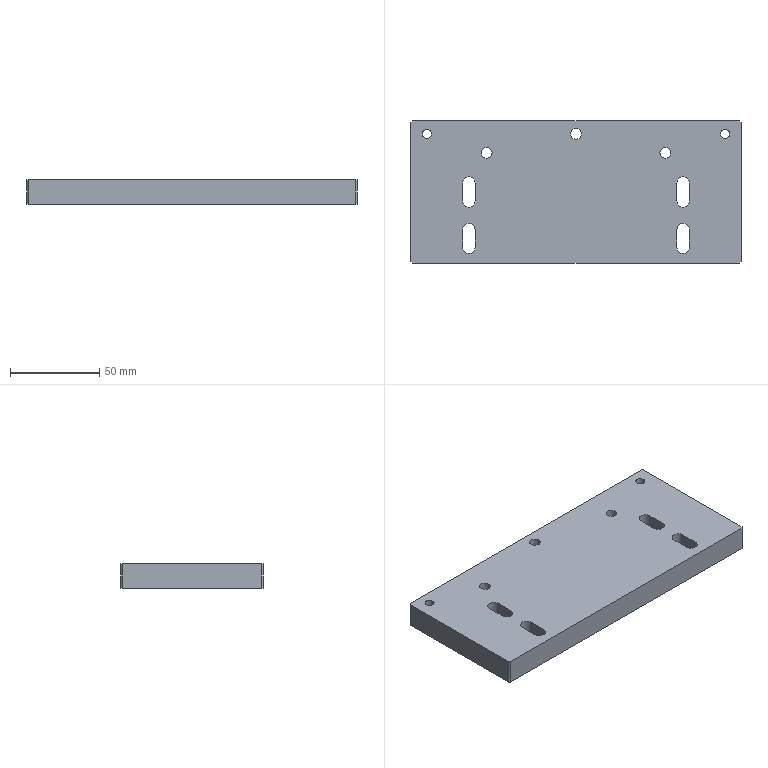Part | NX | 1 solid | 31 faces | box 185 x 80 x 14 mm | volume 199360 mm3 | plane 18 | cylinder 13 | commonest cylinder face diameters 7 x8 6 x3 5 x2
STEP:
#1=CARTESIAN_POINT('',(-91.5,40.,7.));
#2=VERTEX_POINT('',#1);
#3=CARTESIAN_POINT('',(-92.5,39.,7.));
#4=VERTEX_POINT('',#3);
#5=CARTESIAN_POINT('',(-65.75,65.75,7.));
#6=DIRECTION('',(-0.7071,-0.7071,0.));
#7=VECTOR('',#6,1000.);
#8=LINE('',#5,#7);
#9=EDGE_CURVE('',#2,#4,#8,.T.);
#10=ORIENTED_EDGE('',*,*,#9,.F.);
#11=CARTESIAN_POINT('',(-91.5,40.,-7.));
#12=VERTEX_POINT('',#11);
#13=CARTESIAN_POINT('',(-91.5,40.,7.));
#14=DIRECTION('',(0.,0.,1.));
#15=VECTOR('',#14,1000.);
#16=LINE('',#13,#15);
#17=EDGE_CURVE('',#12,#2,#16,.T.);
#18=ORIENTED_EDGE('',*,*,#17,.F.);
#19=CARTESIAN_POINT('',(-92.5,39.,-7.));
#20=VERTEX_POINT('',#19);
#21=CARTESIAN_POINT('',(-92.5,39.,-7.));
#22=DIRECTION('',(0.7071,0.7071,0.));
#23=VECTOR('',#22,1000.);
#24=LINE('',#21,#23);
#25=EDGE_CURVE('',#20,#12,#24,.T.);
#26=ORIENTED_EDGE('',*,*,#25,.F.);
#27=CARTESIAN_POINT('',(-92.5,39.,7.));
#28=DIRECTION('',(0.,0.,-1.));
#29=VECTOR('',#28,1000.);
#30=LINE('',#27,#29);
#31=EDGE_CURVE('',#4,#20,#30,.T.);
#32=ORIENTED_EDGE('',*,*,#31,.F.);
#33=EDGE_LOOP('',(#10,#18,#26,#32));
#34=FACE_BOUND('',#33,.T.);
#35=CARTESIAN_POINT('',(-92.5,39.,7.));
#36=DIRECTION('',(0.7071,-0.7071,0.));
#37=DIRECTION('',(0.,0.,-1.));
#38=AXIS2_PLACEMENT_3D('',#35,#36,#37);
#39=PLANE('',#38);
#40=ADVANCED_FACE('',(#34),#39,.F.);
#41=CARTESIAN_POINT('',(-92.5,-39.,7.));
#42=VERTEX_POINT('',#41);
#43=CARTESIAN_POINT('',(-91.5,-40.,7.));
#44=VERTEX_POINT('',#43);
#45=CARTESIAN_POINT('',(-65.75,-65.75,7.));
#46=DIRECTION('',(0.7071,-0.7071,0.));
#47=VECTOR('',#46,1000.);
#48=LINE('',#45,#47);
#49=EDGE_CURVE('',#42,#44,#48,.T.);
#50=ORIENTED_EDGE('',*,*,#49,.F.);
#51=CARTESIAN_POINT('',(-92.5,-39.,-7.));
#52=VERTEX_POINT('',#51);
#53=CARTESIAN_POINT('',(-92.5,-39.,7.));
#54=DIRECTION('',(0.,0.,1.));
#55=VECTOR('',#54,1000.);
#56=LINE('',#53,#55);
#57=EDGE_CURVE('',#52,#42,#56,.T.);
#58=ORIENTED_EDGE('',*,*,#57,.F.);
#59=CARTESIAN_POINT('',(-91.5,-40.,-7.));
#60=VERTEX_POINT('',#59);
#61=CARTESIAN_POINT('',(-91.5,-40.,-7.));
#62=DIRECTION('',(-0.7071,0.7071,0.));
#63=VECTOR('',#62,1000.);
#64=LINE('',#61,#63);
#65=EDGE_CURVE('',#60,#52,#64,.T.);
#66=ORIENTED_EDGE('',*,*,#65,.F.);
#67=CARTESIAN_POINT('',(-91.5,-40.,7.));
#68=DIRECTION('',(0.,0.,-1.));
#69=VECTOR('',#68,1000.);
#70=LINE('',#67,#69);
#71=EDGE_CURVE('',#44,#60,#70,.T.);
#72=ORIENTED_EDGE('',*,*,#71,.F.);
#73=EDGE_LOOP('',(#50,#58,#66,#72));
#74=FACE_BOUND('',#73,.T.);
#75=CARTESIAN_POINT('',(-91.5,-40.,7.));
#76=DIRECTION('',(0.7071,0.7071,0.));
#77=DIRECTION('',(0.,0.,-1.));
#78=AXIS2_PLACEMENT_3D('',#75,#76,#77);
#79=PLANE('',#78);
#80=ADVANCED_FACE('',(#74),#79,.F.);
#81=CARTESIAN_POINT('',(91.5,-40.,7.));
#82=VERTEX_POINT('',#81);
#83=CARTESIAN_POINT('',(92.5,-39.,7.));
#84=VERTEX_POINT('',#83);
#85=CARTESIAN_POINT('',(65.75,-65.75,7.));
#86=DIRECTION('',(0.7071,0.7071,0.));
#87=VECTOR('',#86,1000.);
#88=LINE('',#85,#87);
#89=EDGE_CURVE('',#82,#84,#88,.T.);
#90=ORIENTED_EDGE('',*,*,#89,.F.);
#91=CARTESIAN_POINT('',(91.5,-40.,-7.));
#92=VERTEX_POINT('',#91);
#93=CARTESIAN_POINT('',(91.5,-40.,7.));
#94=DIRECTION('',(0.,0.,1.));
#95=VECTOR('',#94,1000.);
#96=LINE('',#93,#95);
#97=EDGE_CURVE('',#92,#82,#96,.T.);
#98=ORIENTED_EDGE('',*,*,#97,.F.);
#99=CARTESIAN_POINT('',(92.5,-39.,-7.));
#100=VERTEX_POINT('',#99);
#101=CARTESIAN_POINT('',(92.5,-39.,-7.));
#102=DIRECTION('',(-0.7071,-0.7071,0.));
#103=VECTOR('',#102,1000.);
#104=LINE('',#101,#103);
#105=EDGE_CURVE('',#100,#92,#104,.T.);
#106=ORIENTED_EDGE('',*,*,#105,.F.);
#107=CARTESIAN_POINT('',(92.5,-39.,7.));
#108=DIRECTION('',(0.,0.,-1.));
#109=VECTOR('',#108,1000.);
#110=LINE('',#107,#109);
#111=EDGE_CURVE('',#84,#100,#110,.T.);
#112=ORIENTED_EDGE('',*,*,#111,.F.);
#113=EDGE_LOOP('',(#90,#98,#106,#112));
#114=FACE_BOUND('',#113,.T.);
#115=CARTESIAN_POINT('',(92.5,-39.,7.));
#116=DIRECTION('',(-0.7071,0.7071,0.));
#117=DIRECTION('',(0.,0.,-1.));
#118=AXIS2_PLACEMENT_3D('',#115,#116,#117);
#119=PLANE('',#118);
#120=ADVANCED_FACE('',(#114),#119,.F.);
#121=CARTESIAN_POINT('',(92.5,39.,7.));
#122=VERTEX_POINT('',#121);
#123=CARTESIAN_POINT('',(91.5,40.,7.));
#124=VERTEX_POINT('',#123);
#125=CARTESIAN_POINT('',(65.75,65.75,7.));
#126=DIRECTION('',(-0.7071,0.7071,0.));
#127=VECTOR('',#126,1000.);
#128=LINE('',#125,#127);
#129=EDGE_CURVE('',#122,#124,#128,.T.);
#130=ORIENTED_EDGE('',*,*,#129,.F.);
#131=CARTESIAN_POINT('',(92.5,39.,-7.));
#132=VERTEX_POINT('',#131);
#133=CARTESIAN_POINT('',(92.5,39.,7.));
#134=DIRECTION('',(0.,0.,1.));
#135=VECTOR('',#134,1000.);
#136=LINE('',#133,#135);
#137=EDGE_CURVE('',#132,#122,#136,.T.);
#138=ORIENTED_EDGE('',*,*,#137,.F.);
#139=CARTESIAN_POINT('',(91.5,40.,-7.));
#140=VERTEX_POINT('',#139);
#141=CARTESIAN_POINT('',(91.5,40.,-7.));
#142=DIRECTION('',(0.7071,-0.7071,0.));
#143=VECTOR('',#142,1000.);
#144=LINE('',#141,#143);
#145=EDGE_CURVE('',#140,#132,#144,.T.);
#146=ORIENTED_EDGE('',*,*,#145,.F.);
#147=CARTESIAN_POINT('',(91.5,40.,7.));
#148=DIRECTION('',(0.,0.,-1.));
#149=VECTOR('',#148,1000.);
#150=LINE('',#147,#149);
#151=EDGE_CURVE('',#124,#140,#150,.T.);
#152=ORIENTED_EDGE('',*,*,#151,.F.);
#153=EDGE_LOOP('',(#130,#138,#146,#152));
#154=FACE_BOUND('',#153,.T.);
#155=CARTESIAN_POINT('',(91.5,40.,7.));
#156=DIRECTION('',(-0.7071,-0.7071,0.));
#157=DIRECTION('',(0.,0.,-1.));
#158=AXIS2_PLACEMENT_3D('',#155,#156,#157);
#159=PLANE('',#158);
#160=ADVANCED_FACE('',(#154),#159,.F.);
#161=CARTESIAN_POINT('',(-56.5,-21.,7.));
#162=VERTEX_POINT('',#161);
#163=CARTESIAN_POINT('',(-56.5,-21.,-7.));
#164=VERTEX_POINT('',#163);
#165=CARTESIAN_POINT('',(-56.5,-21.,7.));
#166=DIRECTION('',(0.,0.,-1.));
#167=VECTOR('',#166,1000.);
#168=LINE('',#165,#167);
#169=EDGE_CURVE('',#162,#164,#168,.T.);
#170=ORIENTED_EDGE('',*,*,#169,.T.);
#171=CARTESIAN_POINT('',(-56.5,-31.,-7.));
#172=VERTEX_POINT('',#171);
#173=CARTESIAN_POINT('',(-56.5,0.,-7.));
#174=DIRECTION('',(0.,1.,0.));
#175=VECTOR('',#174,1000.);
#176=LINE('',#173,#175);
#177=EDGE_CURVE('',#172,#164,#176,.T.);
#178=ORIENTED_EDGE('',*,*,#177,.F.);
#179=CARTESIAN_POINT('',(-56.5,-31.,7.));
#180=VERTEX_POINT('',#179);
#181=CARTESIAN_POINT('',(-56.5,-31.,7.));
#182=DIRECTION('',(0.,0.,-1.));
#183=VECTOR('',#182,1000.);
#184=LINE('',#181,#183);
#185=EDGE_CURVE('',#180,#172,#184,.T.);
#186=ORIENTED_EDGE('',*,*,#185,.F.);
#187=CARTESIAN_POINT('',(-56.5,-5.,7.));
#188=DIRECTION('',(0.,1.,0.));
#189=VECTOR('',#188,1000.);
#190=LINE('',#187,#189);
#191=EDGE_CURVE('',#180,#162,#190,.T.);
#192=ORIENTED_EDGE('',*,*,#191,.T.);
#193=EDGE_LOOP('',(#170,#178,#186,#192));
#194=FACE_BOUND('',#193,.T.);
#195=CARTESIAN_POINT('',(-56.5,-5.,-7.));
#196=DIRECTION('',(1.,0.,0.));
#197=DIRECTION('',(0.,0.,-1.));
#198=AXIS2_PLACEMENT_3D('',#195,#196,#197);
#199=PLANE('',#198);
#200=ADVANCED_FACE('',(#194),#199,.F.);
#201=CARTESIAN_POINT('',(-63.5,-21.,-7.));
#202=VERTEX_POINT('',#201);
#203=CARTESIAN_POINT('',(-63.5,-21.,7.));
#204=VERTEX_POINT('',#203);
#205=CARTESIAN_POINT('',(-63.5,-21.,7.));
#206=DIRECTION('',(0.,0.,1.));
#207=VECTOR('',#206,1000.);
#208=LINE('',#205,#207);
#209=EDGE_CURVE('',#202,#204,#208,.T.);
#210=ORIENTED_EDGE('',*,*,#209,.T.);
#211=CARTESIAN_POINT('',(-63.5,-31.,7.));
#212=VERTEX_POINT('',#211);
#213=CARTESIAN_POINT('',(-63.5,0.,7.));
#214=DIRECTION('',(0.,1.,0.));
#215=VECTOR('',#214,1000.);
#216=LINE('',#213,#215);
#217=EDGE_CURVE('',#212,#204,#216,.T.);
#218=ORIENTED_EDGE('',*,*,#217,.F.);
#219=CARTESIAN_POINT('',(-63.5,-31.,-7.));
#220=VERTEX_POINT('',#219);
#221=CARTESIAN_POINT('',(-63.5,-31.,7.));
#222=DIRECTION('',(0.,0.,-1.));
#223=VECTOR('',#222,1000.);
#224=LINE('',#221,#223);
#225=EDGE_CURVE('',#212,#220,#224,.T.);
#226=ORIENTED_EDGE('',*,*,#225,.T.);
#227=CARTESIAN_POINT('',(-63.5,-5.,-7.));
#228=DIRECTION('',(0.,1.,0.));
#229=VECTOR('',#228,1000.);
#230=LINE('',#227,#229);
#231=EDGE_CURVE('',#220,#202,#230,.T.);
#232=ORIENTED_EDGE('',*,*,#231,.T.);
#233=EDGE_LOOP('',(#210,#218,#226,#232));
#234=FACE_BOUND('',#233,.T.);
#235=CARTESIAN_POINT('',(-63.5,-5.,7.));
#236=DIRECTION('',(-1.,0.,0.));
#237=DIRECTION('',(0.,0.,1.));
#238=AXIS2_PLACEMENT_3D('',#235,#236,#237);
#239=PLANE('',#238);
#240=ADVANCED_FACE('',(#234),#239,.F.);
#241=CARTESIAN_POINT('',(-60.,-31.,7.));
#242=DIRECTION('',(0.,0.,1.));
#243=DIRECTION('',(1.,0.,0.));
#244=AXIS2_PLACEMENT_3D('',#241,#242,#243);
#245=CIRCLE('',#244,3.5);
#246=EDGE_CURVE('',#212,#180,#245,.T.);
#247=ORIENTED_EDGE('',*,*,#246,.T.);
#248=ORIENTED_EDGE('',*,*,#185,.T.);
#249=CARTESIAN_POINT('',(-60.,-31.,-7.));
#250=DIRECTION('',(0.,0.,1.));
#251=DIRECTION('',(1.,0.,0.));
#252=AXIS2_PLACEMENT_3D('',#249,#250,#251);
#253=CIRCLE('',#252,3.5);
#254=EDGE_CURVE('',#220,#172,#253,.T.);
#255=ORIENTED_EDGE('',*,*,#254,.F.);
#256=ORIENTED_EDGE('',*,*,#225,.F.);
#257=EDGE_LOOP('',(#247,#248,#255,#256));
#258=FACE_BOUND('',#257,.T.);
#259=CARTESIAN_POINT('',(-60.,-31.,7.));
#260=DIRECTION('',(0.,0.,1.));
#261=DIRECTION('',(1.,0.,0.));
#262=AXIS2_PLACEMENT_3D('',#259,#260,#261);
#263=CYLINDRICAL_SURFACE('',#262,3.5);
#264=ADVANCED_FACE('',(#258),#263,.F.);
#265=CARTESIAN_POINT('',(-60.,-21.,-7.));
#266=DIRECTION('',(0.,0.,1.));
#267=DIRECTION('',(1.,0.,0.));
#268=AXIS2_PLACEMENT_3D('',#265,#266,#267);
#269=CIRCLE('',#268,3.5);
#270=EDGE_CURVE('',#164,#202,#269,.T.);
#271=ORIENTED_EDGE('',*,*,#270,.F.);
#272=ORIENTED_EDGE('',*,*,#169,.F.);
#273=CARTESIAN_POINT('',(-60.,-21.,7.));
#274=DIRECTION('',(0.,0.,1.));
#275=DIRECTION('',(1.,0.,0.));
#276=AXIS2_PLACEMENT_3D('',#273,#274,#275);
#277=CIRCLE('',#276,3.5);
#278=EDGE_CURVE('',#162,#204,#277,.T.);
#279=ORIENTED_EDGE('',*,*,#278,.T.);
#280=ORIENTED_EDGE('',*,*,#209,.F.);
#281=EDGE_LOOP('',(#271,#272,#279,#280));
#282=FACE_BOUND('',#281,.T.);
#283=CARTESIAN_POINT('',(-60.,-21.,7.));
#284=DIRECTION('',(0.,0.,1.));
#285=DIRECTION('',(1.,0.,0.));
#286=AXIS2_PLACEMENT_3D('',#283,#284,#285);
#287=CYLINDRICAL_SURFACE('',#286,3.5);
#288=ADVANCED_FACE('',(#282),#287,.F.);
#289=CARTESIAN_POINT('',(-56.5,5.,7.));
#290=VERTEX_POINT('',#289);
#291=CARTESIAN_POINT('',(-56.5,5.,-7.));
#292=VERTEX_POINT('',#291);
#293=CARTESIAN_POINT('',(-56.5,5.,-7.));
#294=DIRECTION('',(0.,0.,-1.));
#295=VECTOR('',#294,1000.);
#296=LINE('',#293,#295);
#297=EDGE_CURVE('',#290,#292,#296,.T.);
#298=ORIENTED_EDGE('',*,*,#297,.T.);
#299=CARTESIAN_POINT('',(-56.5,-5.,-7.));
#300=VERTEX_POINT('',#299);
#301=CARTESIAN_POINT('',(-56.5,-5.,-7.));
#302=DIRECTION('',(0.,1.,0.));
#303=VECTOR('',#302,1000.);
#304=LINE('',#301,#303);
#305=EDGE_CURVE('',#300,#292,#304,.T.);
#306=ORIENTED_EDGE('',*,*,#305,.F.);
#307=CARTESIAN_POINT('',(-56.5,-5.,7.));
#308=VERTEX_POINT('',#307);
#309=CARTESIAN_POINT('',(-56.5,-5.,-7.));
#310=DIRECTION('',(0.,0.,-1.));
#311=VECTOR('',#310,1000.);
#312=LINE('',#309,#311);
#313=EDGE_CURVE('',#308,#300,#312,.T.);
#314=ORIENTED_EDGE('',*,*,#313,.F.);
#315=CARTESIAN_POINT('',(-56.5,-5.,7.));
#316=DIRECTION('',(0.,1.,0.));
#317=VECTOR('',#316,1000.);
#318=LINE('',#315,#317);
#319=EDGE_CURVE('',#308,#290,#318,.T.);
#320=ORIENTED_EDGE('',*,*,#319,.T.);
#321=EDGE_LOOP('',(#298,#306,#314,#320));
#322=FACE_BOUND('',#321,.T.);
#323=CARTESIAN_POINT('',(-56.5,-5.,-7.));
#324=DIRECTION('',(1.,0.,0.));
#325=DIRECTION('',(0.,0.,-1.));
#326=AXIS2_PLACEMENT_3D('',#323,#324,#325);
#327=PLANE('',#326);
#328=ADVANCED_FACE('',(#322),#327,.F.);
#329=CARTESIAN_POINT('',(-63.5,5.,-7.));
#330=VERTEX_POINT('',#329);
#331=CARTESIAN_POINT('',(-63.5,5.,7.));
#332=VERTEX_POINT('',#331);
#333=CARTESIAN_POINT('',(-63.5,5.,7.));
#334=DIRECTION('',(0.,0.,1.));
#335=VECTOR('',#334,1000.);
#336=LINE('',#333,#335);
#337=EDGE_CURVE('',#330,#332,#336,.T.);
#338=ORIENTED_EDGE('',*,*,#337,.T.);
#339=CARTESIAN_POINT('',(-63.5,-5.,7.));
#340=VERTEX_POINT('',#339);
#341=CARTESIAN_POINT('',(-63.5,-5.,7.));
#342=DIRECTION('',(0.,1.,0.));
#343=VECTOR('',#342,1000.);
#344=LINE('',#341,#343);
#345=EDGE_CURVE('',#340,#332,#344,.T.);
#346=ORIENTED_EDGE('',*,*,#345,.F.);
#347=CARTESIAN_POINT('',(-63.5,-5.,-7.));
#348=VERTEX_POINT('',#347);
#349=CARTESIAN_POINT('',(-63.5,-5.,7.));
#350=DIRECTION('',(0.,0.,-1.));
#351=VECTOR('',#350,1000.);
#352=LINE('',#349,#351);
#353=EDGE_CURVE('',#340,#348,#352,.T.);
#354=ORIENTED_EDGE('',*,*,#353,.T.);
#355=CARTESIAN_POINT('',(-63.5,-5.,-7.));
#356=DIRECTION('',(0.,1.,0.));
#357=VECTOR('',#356,1000.);
#358=LINE('',#355,#357);
#359=EDGE_CURVE('',#348,#330,#358,.T.);
#360=ORIENTED_EDGE('',*,*,#359,.T.);
#361=EDGE_LOOP('',(#338,#346,#354,#360));
#362=FACE_BOUND('',#361,.T.);
#363=CARTESIAN_POINT('',(-63.5,-5.,7.));
#364=DIRECTION('',(-1.,0.,0.));
#365=DIRECTION('',(0.,0.,1.));
#366=AXIS2_PLACEMENT_3D('',#363,#364,#365);
#367=PLANE('',#366);
#368=ADVANCED_FACE('',(#362),#367,.F.);
#369=CARTESIAN_POINT('',(-60.,-5.,7.));
#370=DIRECTION('',(0.,0.,1.));
#371=DIRECTION('',(1.,0.,0.));
#372=AXIS2_PLACEMENT_3D('',#369,#370,#371);
#373=CIRCLE('',#372,3.5);
#374=EDGE_CURVE('',#340,#308,#373,.T.);
#375=ORIENTED_EDGE('',*,*,#374,.T.);
#376=ORIENTED_EDGE('',*,*,#313,.T.);
#377=CARTESIAN_POINT('',(-60.,-5.,-7.));
#378=DIRECTION('',(0.,0.,1.));
#379=DIRECTION('',(1.,0.,0.));
#380=AXIS2_PLACEMENT_3D('',#377,#378,#379);
#381=CIRCLE('',#380,3.5);
#382=EDGE_CURVE('',#348,#300,#381,.T.);
#383=ORIENTED_EDGE('',*,*,#382,.F.);
#384=ORIENTED_EDGE('',*,*,#353,.F.);
#385=EDGE_LOOP('',(#375,#376,#383,#384));
#386=FACE_BOUND('',#385,.T.);
#387=CARTESIAN_POINT('',(-60.,-5.,7.));
#388=DIRECTION('',(0.,0.,1.));
#389=DIRECTION('',(1.,0.,0.));
#390=AXIS2_PLACEMENT_3D('',#387,#388,#389);
#391=CYLINDRICAL_SURFACE('',#390,3.5);
#392=ADVANCED_FACE('',(#386),#391,.F.);
#393=CARTESIAN_POINT('',(-60.,5.,-7.));
#394=DIRECTION('',(0.,0.,1.));
#395=DIRECTION('',(1.,0.,0.));
#396=AXIS2_PLACEMENT_3D('',#393,#394,#395);
#397=CIRCLE('',#396,3.5);
#398=EDGE_CURVE('',#292,#330,#397,.T.);
#399=ORIENTED_EDGE('',*,*,#398,.F.);
#400=ORIENTED_EDGE('',*,*,#297,.F.);
#401=CARTESIAN_POINT('',(-60.,5.,7.));
#402=DIRECTION('',(0.,0.,1.));
#403=DIRECTION('',(1.,0.,0.));
#404=AXIS2_PLACEMENT_3D('',#401,#402,#403);
#405=CIRCLE('',#404,3.5);
#406=EDGE_CURVE('',#290,#332,#405,.T.);
#407=ORIENTED_EDGE('',*,*,#406,.T.);
#408=ORIENTED_EDGE('',*,*,#337,.F.);
#409=EDGE_LOOP('',(#399,#400,#407,#408));
#410=FACE_BOUND('',#409,.T.);
#411=CARTESIAN_POINT('',(-60.,5.,7.));
#412=DIRECTION('',(0.,0.,1.));
#413=DIRECTION('',(1.,0.,0.));
#414=AXIS2_PLACEMENT_3D('',#411,#412,#413);
#415=CYLINDRICAL_SURFACE('',#414,3.5);
#416=ADVANCED_FACE('',(#410),#415,.F.);
#417=CARTESIAN_POINT('',(63.5,-21.,7.));
#418=VERTEX_POINT('',#417);
#419=CARTESIAN_POINT('',(63.5,-21.,-7.));
#420=VERTEX_POINT('',#419);
#421=CARTESIAN_POINT('',(63.5,-21.,7.));
#422=DIRECTION('',(0.,0.,-1.));
#423=VECTOR('',#422,1000.);
#424=LINE('',#421,#423);
#425=EDGE_CURVE('',#418,#420,#424,.T.);
#426=ORIENTED_EDGE('',*,*,#425,.T.);
#427=CARTESIAN_POINT('',(63.5,-31.,-7.));
#428=VERTEX_POINT('',#427);
#429=CARTESIAN_POINT('',(63.5,0.,-7.));
#430=DIRECTION('',(0.,1.,0.));
#431=VECTOR('',#430,1000.);
#432=LINE('',#429,#431);
#433=EDGE_CURVE('',#428,#420,#432,.T.);
#434=ORIENTED_EDGE('',*,*,#433,.F.);
#435=CARTESIAN_POINT('',(63.5,-31.,7.));
#436=VERTEX_POINT('',#435);
#437=CARTESIAN_POINT('',(63.5,-31.,7.));
#438=DIRECTION('',(0.,0.,-1.));
#439=VECTOR('',#438,1000.);
#440=LINE('',#437,#439);
#441=EDGE_CURVE('',#436,#428,#440,.T.);
#442=ORIENTED_EDGE('',*,*,#441,.F.);
#443=CARTESIAN_POINT('',(63.5,-5.,7.));
#444=DIRECTION('',(0.,1.,0.));
#445=VECTOR('',#444,1000.);
#446=LINE('',#443,#445);
#447=EDGE_CURVE('',#436,#418,#446,.T.);
#448=ORIENTED_EDGE('',*,*,#447,.T.);
#449=EDGE_LOOP('',(#426,#434,#442,#448));
#450=FACE_BOUND('',#449,.T.);
#451=CARTESIAN_POINT('',(63.5,-5.,-7.));
#452=DIRECTION('',(1.,0.,0.));
#453=DIRECTION('',(0.,0.,-1.));
#454=AXIS2_PLACEMENT_3D('',#451,#452,#453);
#455=PLANE('',#454);
#456=ADVANCED_FACE('',(#450),#455,.F.);
#457=CARTESIAN_POINT('',(56.5,-21.,-7.));
#458=VERTEX_POINT('',#457);
#459=CARTESIAN_POINT('',(56.5,-21.,7.));
#460=VERTEX_POINT('',#459);
#461=CARTESIAN_POINT('',(56.5,-21.,7.));
#462=DIRECTION('',(0.,0.,1.));
#463=VECTOR('',#462,1000.);
#464=LINE('',#461,#463);
#465=EDGE_CURVE('',#458,#460,#464,.T.);
#466=ORIENTED_EDGE('',*,*,#465,.T.);
#467=CARTESIAN_POINT('',(56.5,-31.,7.));
#468=VERTEX_POINT('',#467);
#469=CARTESIAN_POINT('',(56.5,0.,7.));
#470=DIRECTION('',(0.,1.,0.));
#471=VECTOR('',#470,1000.);
#472=LINE('',#469,#471);
#473=EDGE_CURVE('',#468,#460,#472,.T.);
#474=ORIENTED_EDGE('',*,*,#473,.F.);
#475=CARTESIAN_POINT('',(56.5,-31.,-7.));
#476=VERTEX_POINT('',#475);
#477=CARTESIAN_POINT('',(56.5,-31.,7.));
#478=DIRECTION('',(0.,0.,-1.));
#479=VECTOR('',#478,1000.);
#480=LINE('',#477,#479);
#481=EDGE_CURVE('',#468,#476,#480,.T.);
#482=ORIENTED_EDGE('',*,*,#481,.T.);
#483=CARTESIAN_POINT('',(56.5,-5.,-7.));
#484=DIRECTION('',(0.,1.,0.));
#485=VECTOR('',#484,1000.);
#486=LINE('',#483,#485);
#487=EDGE_CURVE('',#476,#458,#486,.T.);
#488=ORIENTED_EDGE('',*,*,#487,.T.);
#489=EDGE_LOOP('',(#466,#474,#482,#488));
#490=FACE_BOUND('',#489,.T.);
#491=CARTESIAN_POINT('',(56.5,-5.,7.));
#492=DIRECTION('',(-1.,0.,0.));
#493=DIRECTION('',(0.,0.,1.));
#494=AXIS2_PLACEMENT_3D('',#491,#492,#493);
#495=PLANE('',#494);
#496=ADVANCED_FACE('',(#490),#495,.F.);
#497=CARTESIAN_POINT('',(60.,-31.,7.));
#498=DIRECTION('',(0.,0.,1.));
#499=DIRECTION('',(1.,0.,0.));
#500=AXIS2_PLACEMENT_3D('',#497,#498,#499);
#501=CIRCLE('',#500,3.5);
#502=EDGE_CURVE('',#468,#436,#501,.T.);
#503=ORIENTED_EDGE('',*,*,#502,.T.);
#504=ORIENTED_EDGE('',*,*,#441,.T.);
#505=CARTESIAN_POINT('',(60.,-31.,-7.));
#506=DIRECTION('',(0.,0.,1.));
#507=DIRECTION('',(1.,0.,0.));
#508=AXIS2_PLACEMENT_3D('',#505,#506,#507);
#509=CIRCLE('',#508,3.5);
#510=EDGE_CURVE('',#476,#428,#509,.T.);
#511=ORIENTED_EDGE('',*,*,#510,.F.);
#512=ORIENTED_EDGE('',*,*,#481,.F.);
#513=EDGE_LOOP('',(#503,#504,#511,#512));
#514=FACE_BOUND('',#513,.T.);
#515=CARTESIAN_POINT('',(60.,-31.,7.));
#516=DIRECTION('',(0.,0.,1.));
#517=DIRECTION('',(1.,0.,0.));
#518=AXIS2_PLACEMENT_3D('',#515,#516,#517);
#519=CYLINDRICAL_SURFACE('',#518,3.5);
#520=ADVANCED_FACE('',(#514),#519,.F.);
#521=CARTESIAN_POINT('',(60.,-21.,-7.));
#522=DIRECTION('',(0.,0.,1.));
#523=DIRECTION('',(1.,0.,0.));
#524=AXIS2_PLACEMENT_3D('',#521,#522,#523);
#525=CIRCLE('',#524,3.5);
#526=EDGE_CURVE('',#420,#458,#525,.T.);
#527=ORIENTED_EDGE('',*,*,#526,.F.);
#528=ORIENTED_EDGE('',*,*,#425,.F.);
#529=CARTESIAN_POINT('',(60.,-21.,7.));
#530=DIRECTION('',(0.,0.,1.));
#531=DIRECTION('',(1.,0.,0.));
#532=AXIS2_PLACEMENT_3D('',#529,#530,#531);
#533=CIRCLE('',#532,3.5);
#534=EDGE_CURVE('',#418,#460,#533,.T.);
#535=ORIENTED_EDGE('',*,*,#534,.T.);
#536=ORIENTED_EDGE('',*,*,#465,.F.);
#537=EDGE_LOOP('',(#527,#528,#535,#536));
#538=FACE_BOUND('',#537,.T.);
#539=CARTESIAN_POINT('',(60.,-21.,7.));
#540=DIRECTION('',(0.,0.,1.));
#541=DIRECTION('',(1.,0.,0.));
#542=AXIS2_PLACEMENT_3D('',#539,#540,#541);
#543=CYLINDRICAL_SURFACE('',#542,3.5);
#544=ADVANCED_FACE('',(#538),#543,.F.);
#545=CARTESIAN_POINT('',(63.5,5.,7.));
#546=VERTEX_POINT('',#545);
#547=CARTESIAN_POINT('',(63.5,5.,-7.));
#548=VERTEX_POINT('',#547);
#549=CARTESIAN_POINT('',(63.5,5.,-7.));
#550=DIRECTION('',(0.,0.,-1.));
#551=VECTOR('',#550,1000.);
#552=LINE('',#549,#551);
#553=EDGE_CURVE('',#546,#548,#552,.T.);
#554=ORIENTED_EDGE('',*,*,#553,.T.);
#555=CARTESIAN_POINT('',(63.5,-5.,-7.));
#556=VERTEX_POINT('',#555);
#557=CARTESIAN_POINT('',(63.5,-5.,-7.));
#558=DIRECTION('',(0.,1.,0.));
#559=VECTOR('',#558,1000.);
#560=LINE('',#557,#559);
#561=EDGE_CURVE('',#556,#548,#560,.T.);
#562=ORIENTED_EDGE('',*,*,#561,.F.);
#563=CARTESIAN_POINT('',(63.5,-5.,7.));
#564=VERTEX_POINT('',#563);
#565=CARTESIAN_POINT('',(63.5,-5.,-7.));
#566=DIRECTION('',(0.,0.,-1.));
#567=VECTOR('',#566,1000.);
#568=LINE('',#565,#567);
#569=EDGE_CURVE('',#564,#556,#568,.T.);
#570=ORIENTED_EDGE('',*,*,#569,.F.);
#571=CARTESIAN_POINT('',(63.5,-5.,7.));
#572=DIRECTION('',(0.,1.,0.));
#573=VECTOR('',#572,1000.);
#574=LINE('',#571,#573);
#575=EDGE_CURVE('',#564,#546,#574,.T.);
#576=ORIENTED_EDGE('',*,*,#575,.T.);
#577=EDGE_LOOP('',(#554,#562,#570,#576));
#578=FACE_BOUND('',#577,.T.);
#579=CARTESIAN_POINT('',(63.5,-5.,-7.));
#580=DIRECTION('',(1.,0.,0.));
#581=DIRECTION('',(0.,0.,-1.));
#582=AXIS2_PLACEMENT_3D('',#579,#580,#581);
#583=PLANE('',#582);
#584=ADVANCED_FACE('',(#578),#583,.F.);
#585=CARTESIAN_POINT('',(56.5,5.,-7.));
#586=VERTEX_POINT('',#585);
#587=CARTESIAN_POINT('',(56.5,5.,7.));
#588=VERTEX_POINT('',#587);
#589=CARTESIAN_POINT('',(56.5,5.,7.));
#590=DIRECTION('',(0.,0.,1.));
#591=VECTOR('',#590,1000.);
#592=LINE('',#589,#591);
#593=EDGE_CURVE('',#586,#588,#592,.T.);
#594=ORIENTED_EDGE('',*,*,#593,.T.);
#595=CARTESIAN_POINT('',(56.5,-5.,7.));
#596=VERTEX_POINT('',#595);
#597=CARTESIAN_POINT('',(56.5,-5.,7.));
#598=DIRECTION('',(0.,1.,0.));
#599=VECTOR('',#598,1000.);
#600=LINE('',#597,#599);
#601=EDGE_CURVE('',#596,#588,#600,.T.);
#602=ORIENTED_EDGE('',*,*,#601,.F.);
#603=CARTESIAN_POINT('',(56.5,-5.,-7.));
#604=VERTEX_POINT('',#603);
#605=CARTESIAN_POINT('',(56.5,-5.,7.));
#606=DIRECTION('',(0.,0.,-1.));
#607=VECTOR('',#606,1000.);
#608=LINE('',#605,#607);
#609=EDGE_CURVE('',#596,#604,#608,.T.);
#610=ORIENTED_EDGE('',*,*,#609,.T.);
#611=CARTESIAN_POINT('',(56.5,-5.,-7.));
#612=DIRECTION('',(0.,1.,0.));
#613=VECTOR('',#612,1000.);
#614=LINE('',#611,#613);
#615=EDGE_CURVE('',#604,#586,#614,.T.);
#616=ORIENTED_EDGE('',*,*,#615,.T.);
#617=EDGE_LOOP('',(#594,#602,#610,#616));
#618=FACE_BOUND('',#617,.T.);
#619=CARTESIAN_POINT('',(56.5,-5.,7.));
#620=DIRECTION('',(-1.,0.,0.));
#621=DIRECTION('',(0.,0.,1.));
#622=AXIS2_PLACEMENT_3D('',#619,#620,#621);
#623=PLANE('',#622);
#624=ADVANCED_FACE('',(#618),#623,.F.);
#625=CARTESIAN_POINT('',(60.,-5.,7.));
#626=DIRECTION('',(0.,0.,1.));
#627=DIRECTION('',(1.,0.,0.));
#628=AXIS2_PLACEMENT_3D('',#625,#626,#627);
#629=CIRCLE('',#628,3.5);
#630=EDGE_CURVE('',#596,#564,#629,.T.);
#631=ORIENTED_EDGE('',*,*,#630,.T.);
#632=ORIENTED_EDGE('',*,*,#569,.T.);
#633=CARTESIAN_POINT('',(60.,-5.,-7.));
#634=DIRECTION('',(0.,0.,1.));
#635=DIRECTION('',(1.,0.,0.));
#636=AXIS2_PLACEMENT_3D('',#633,#634,#635);
#637=CIRCLE('',#636,3.5);
#638=EDGE_CURVE('',#604,#556,#637,.T.);
#639=ORIENTED_EDGE('',*,*,#638,.F.);
#640=ORIENTED_EDGE('',*,*,#609,.F.);
#641=EDGE_LOOP('',(#631,#632,#639,#640));
#642=FACE_BOUND('',#641,.T.);
#643=CARTESIAN_POINT('',(60.,-5.,7.));
#644=DIRECTION('',(0.,0.,1.));
#645=DIRECTION('',(1.,0.,0.));
#646=AXIS2_PLACEMENT_3D('',#643,#644,#645);
#647=CYLINDRICAL_SURFACE('',#646,3.5);
#648=ADVANCED_FACE('',(#642),#647,.F.);
#649=CARTESIAN_POINT('',(60.,5.,-7.));
#650=DIRECTION('',(0.,0.,1.));
#651=DIRECTION('',(1.,0.,0.));
#652=AXIS2_PLACEMENT_3D('',#649,#650,#651);
#653=CIRCLE('',#652,3.5);
#654=EDGE_CURVE('',#548,#586,#653,.T.);
#655=ORIENTED_EDGE('',*,*,#654,.F.);
#656=ORIENTED_EDGE('',*,*,#553,.F.);
#657=CARTESIAN_POINT('',(60.,5.,7.));
#658=DIRECTION('',(0.,0.,1.));
#659=DIRECTION('',(1.,0.,0.));
#660=AXIS2_PLACEMENT_3D('',#657,#658,#659);
#661=CIRCLE('',#660,3.5);
#662=EDGE_CURVE('',#546,#588,#661,.T.);
#663=ORIENTED_EDGE('',*,*,#662,.T.);
#664=ORIENTED_EDGE('',*,*,#593,.F.);
#665=EDGE_LOOP('',(#655,#656,#663,#664));
#666=FACE_BOUND('',#665,.T.);
#667=CARTESIAN_POINT('',(60.,5.,7.));
#668=DIRECTION('',(0.,0.,1.));
#669=DIRECTION('',(1.,0.,0.));
#670=AXIS2_PLACEMENT_3D('',#667,#668,#669);
#671=CYLINDRICAL_SURFACE('',#670,3.5);
#672=ADVANCED_FACE('',(#666),#671,.F.);
#673=CARTESIAN_POINT('',(-92.5,40.,-7.));
#674=DIRECTION('',(-1.,0.,0.));
#675=VECTOR('',#674,1000.);
#676=LINE('',#673,#675);
#677=EDGE_CURVE('',#140,#12,#676,.T.);
#678=ORIENTED_EDGE('',*,*,#677,.F.);
#679=ORIENTED_EDGE('',*,*,#145,.T.);
#680=CARTESIAN_POINT('',(92.5,40.,-7.));
#681=DIRECTION('',(0.,1.,0.));
#682=VECTOR('',#681,1000.);
#683=LINE('',#680,#682);
#684=EDGE_CURVE('',#100,#132,#683,.T.);
#685=ORIENTED_EDGE('',*,*,#684,.F.);
#686=ORIENTED_EDGE('',*,*,#105,.T.);
#687=CARTESIAN_POINT('',(-92.5,-40.,-7.));
#688=DIRECTION('',(1.,0.,0.));
#689=VECTOR('',#688,1000.);
#690=LINE('',#687,#689);
#691=EDGE_CURVE('',#60,#92,#690,.T.);
#692=ORIENTED_EDGE('',*,*,#691,.F.);
#693=ORIENTED_EDGE('',*,*,#65,.T.);
#694=CARTESIAN_POINT('',(-92.5,40.,-7.));
#695=DIRECTION('',(0.,-1.,0.));
#696=VECTOR('',#695,1000.);
#697=LINE('',#694,#696);
#698=EDGE_CURVE('',#20,#52,#697,.T.);
#699=ORIENTED_EDGE('',*,*,#698,.F.);
#700=ORIENTED_EDGE('',*,*,#25,.T.);
#701=EDGE_LOOP('',(#678,#679,#685,#686,#692,#693,#699,#700));
#702=FACE_BOUND('',#701,.T.);
#703=CARTESIAN_POINT('',(-81.,32.5,-7.));
#704=VERTEX_POINT('',#703);
#705=CARTESIAN_POINT('',(-83.5,32.5,-7.));
#706=DIRECTION('',(0.,0.,1.));
#707=DIRECTION('',(1.,0.,0.));
#708=AXIS2_PLACEMENT_3D('',#705,#706,#707);
#709=CIRCLE('',#708,2.5);
#710=EDGE_CURVE('',#704,#704,#709,.T.);
#711=ORIENTED_EDGE('',*,*,#710,.T.);
#712=EDGE_LOOP('',(#711));
#713=FACE_BOUND('',#712,.T.);
#714=CARTESIAN_POINT('',(86.,32.5,-7.));
#715=VERTEX_POINT('',#714);
#716=CARTESIAN_POINT('',(83.5,32.5,-7.));
#717=DIRECTION('',(0.,0.,1.));
#718=DIRECTION('',(1.,0.,0.));
#719=AXIS2_PLACEMENT_3D('',#716,#717,#718);
#720=CIRCLE('',#719,2.5);
#721=EDGE_CURVE('',#715,#715,#720,.T.);
#722=ORIENTED_EDGE('',*,*,#721,.T.);
#723=EDGE_LOOP('',(#722));
#724=FACE_BOUND('',#723,.T.);
#725=CARTESIAN_POINT('',(3.,32.5,-7.));
#726=VERTEX_POINT('',#725);
#727=CARTESIAN_POINT('',(0.,32.5,-7.));
#728=DIRECTION('',(0.,0.,1.));
#729=DIRECTION('',(1.,0.,0.));
#730=AXIS2_PLACEMENT_3D('',#727,#728,#729);
#731=CIRCLE('',#730,3.);
#732=EDGE_CURVE('',#726,#726,#731,.T.);
#733=ORIENTED_EDGE('',*,*,#732,.T.);
#734=EDGE_LOOP('',(#733));
#735=FACE_BOUND('',#734,.T.);
#736=CARTESIAN_POINT('',(53.,22.,-7.));
#737=VERTEX_POINT('',#736);
#738=CARTESIAN_POINT('',(50.,22.,-7.));
#739=DIRECTION('',(0.,0.,1.));
#740=DIRECTION('',(1.,0.,0.));
#741=AXIS2_PLACEMENT_3D('',#738,#739,#740);
#742=CIRCLE('',#741,3.);
#743=EDGE_CURVE('',#737,#737,#742,.T.);
#744=ORIENTED_EDGE('',*,*,#743,.T.);
#745=EDGE_LOOP('',(#744));
#746=FACE_BOUND('',#745,.T.);
#747=CARTESIAN_POINT('',(-47.,22.,-7.));
#748=VERTEX_POINT('',#747);
#749=CARTESIAN_POINT('',(-50.,22.,-7.));
#750=DIRECTION('',(0.,0.,1.));
#751=DIRECTION('',(1.,0.,0.));
#752=AXIS2_PLACEMENT_3D('',#749,#750,#751);
#753=CIRCLE('',#752,3.);
#754=EDGE_CURVE('',#748,#748,#753,.T.);
#755=ORIENTED_EDGE('',*,*,#754,.T.);
#756=EDGE_LOOP('',(#755));
#757=FACE_BOUND('',#756,.T.);
#758=ORIENTED_EDGE('',*,*,#615,.F.);
#759=ORIENTED_EDGE('',*,*,#638,.T.);
#760=ORIENTED_EDGE('',*,*,#561,.T.);
#761=ORIENTED_EDGE('',*,*,#654,.T.);
#762=EDGE_LOOP('',(#758,#759,#760,#761));
#763=FACE_BOUND('',#762,.T.);
#764=ORIENTED_EDGE('',*,*,#433,.T.);
#765=ORIENTED_EDGE('',*,*,#526,.T.);
#766=ORIENTED_EDGE('',*,*,#487,.F.);
#767=ORIENTED_EDGE('',*,*,#510,.T.);
#768=EDGE_LOOP('',(#764,#765,#766,#767));
#769=FACE_BOUND('',#768,.T.);
#770=ORIENTED_EDGE('',*,*,#359,.F.);
#771=ORIENTED_EDGE('',*,*,#382,.T.);
#772=ORIENTED_EDGE('',*,*,#305,.T.);
#773=ORIENTED_EDGE('',*,*,#398,.T.);
#774=EDGE_LOOP('',(#770,#771,#772,#773));
#775=FACE_BOUND('',#774,.T.);
#776=ORIENTED_EDGE('',*,*,#254,.T.);
#777=ORIENTED_EDGE('',*,*,#177,.T.);
#778=ORIENTED_EDGE('',*,*,#270,.T.);
#779=ORIENTED_EDGE('',*,*,#231,.F.);
#780=EDGE_LOOP('',(#776,#777,#778,#779));
#781=FACE_BOUND('',#780,.T.);
#782=CARTESIAN_POINT('',(0.,0.,-7.));
#783=DIRECTION('',(0.,0.,1.));
#784=DIRECTION('',(1.,0.,0.));
#785=AXIS2_PLACEMENT_3D('',#782,#783,#784);
#786=PLANE('',#785);
#787=ADVANCED_FACE('',(#702,#713,#724,#735,#746,#757,#763,#769,#775,#781),#786,.F.);
#788=CARTESIAN_POINT('',(92.5,40.,7.));
#789=DIRECTION('',(0.,1.,0.));
#790=VECTOR('',#789,1000.);
#791=LINE('',#788,#790);
#792=EDGE_CURVE('',#84,#122,#791,.T.);
#793=ORIENTED_EDGE('',*,*,#792,.T.);
#794=ORIENTED_EDGE('',*,*,#129,.T.);
#795=CARTESIAN_POINT('',(-92.5,40.,7.));
#796=DIRECTION('',(-1.,0.,0.));
#797=VECTOR('',#796,1000.);
#798=LINE('',#795,#797);
#799=EDGE_CURVE('',#124,#2,#798,.T.);
#800=ORIENTED_EDGE('',*,*,#799,.T.);
#801=ORIENTED_EDGE('',*,*,#9,.T.);
#802=CARTESIAN_POINT('',(-92.5,40.,7.));
#803=DIRECTION('',(0.,-1.,0.));
#804=VECTOR('',#803,1000.);
#805=LINE('',#802,#804);
#806=EDGE_CURVE('',#4,#42,#805,.T.);
#807=ORIENTED_EDGE('',*,*,#806,.T.);
#808=ORIENTED_EDGE('',*,*,#49,.T.);
#809=CARTESIAN_POINT('',(-92.5,-40.,7.));
#810=DIRECTION('',(1.,0.,0.));
#811=VECTOR('',#810,1000.);
#812=LINE('',#809,#811);
#813=EDGE_CURVE('',#44,#82,#812,.T.);
#814=ORIENTED_EDGE('',*,*,#813,.T.);
#815=ORIENTED_EDGE('',*,*,#89,.T.);
#816=EDGE_LOOP('',(#793,#794,#800,#801,#807,#808,#814,#815));
#817=FACE_BOUND('',#816,.T.);
#818=CARTESIAN_POINT('',(-81.,32.5,7.));
#819=VERTEX_POINT('',#818);
#820=CARTESIAN_POINT('',(-83.5,32.5,7.));
#821=DIRECTION('',(0.,0.,1.));
#822=DIRECTION('',(1.,0.,0.));
#823=AXIS2_PLACEMENT_3D('',#820,#821,#822);
#824=CIRCLE('',#823,2.5);
#825=EDGE_CURVE('',#819,#819,#824,.T.);
#826=ORIENTED_EDGE('',*,*,#825,.F.);
#827=EDGE_LOOP('',(#826));
#828=FACE_BOUND('',#827,.T.);
#829=CARTESIAN_POINT('',(86.,32.5,7.));
#830=VERTEX_POINT('',#829);
#831=CARTESIAN_POINT('',(83.5,32.5,7.));
#832=DIRECTION('',(0.,0.,1.));
#833=DIRECTION('',(1.,0.,0.));
#834=AXIS2_PLACEMENT_3D('',#831,#832,#833);
#835=CIRCLE('',#834,2.5);
#836=EDGE_CURVE('',#830,#830,#835,.T.);
#837=ORIENTED_EDGE('',*,*,#836,.F.);
#838=EDGE_LOOP('',(#837));
#839=FACE_BOUND('',#838,.T.);
#840=CARTESIAN_POINT('',(3.,32.5,7.));
#841=VERTEX_POINT('',#840);
#842=CARTESIAN_POINT('',(0.,32.5,7.));
#843=DIRECTION('',(0.,0.,1.));
#844=DIRECTION('',(1.,0.,0.));
#845=AXIS2_PLACEMENT_3D('',#842,#843,#844);
#846=CIRCLE('',#845,3.);
#847=EDGE_CURVE('',#841,#841,#846,.T.);
#848=ORIENTED_EDGE('',*,*,#847,.F.);
#849=EDGE_LOOP('',(#848));
#850=FACE_BOUND('',#849,.T.);
#851=CARTESIAN_POINT('',(53.,22.,7.));
#852=VERTEX_POINT('',#851);
#853=CARTESIAN_POINT('',(50.,22.,7.));
#854=DIRECTION('',(0.,0.,1.));
#855=DIRECTION('',(1.,0.,0.));
#856=AXIS2_PLACEMENT_3D('',#853,#854,#855);
#857=CIRCLE('',#856,3.);
#858=EDGE_CURVE('',#852,#852,#857,.T.);
#859=ORIENTED_EDGE('',*,*,#858,.F.);
#860=EDGE_LOOP('',(#859));
#861=FACE_BOUND('',#860,.T.);
#862=CARTESIAN_POINT('',(-47.,22.,7.));
#863=VERTEX_POINT('',#862);
#864=CARTESIAN_POINT('',(-50.,22.,7.));
#865=DIRECTION('',(0.,0.,1.));
#866=DIRECTION('',(1.,0.,0.));
#867=AXIS2_PLACEMENT_3D('',#864,#865,#866);
#868=CIRCLE('',#867,3.);
#869=EDGE_CURVE('',#863,#863,#868,.T.);
#870=ORIENTED_EDGE('',*,*,#869,.F.);
#871=EDGE_LOOP('',(#870));
#872=FACE_BOUND('',#871,.T.);
#873=ORIENTED_EDGE('',*,*,#601,.T.);
#874=ORIENTED_EDGE('',*,*,#662,.F.);
#875=ORIENTED_EDGE('',*,*,#575,.F.);
#876=ORIENTED_EDGE('',*,*,#630,.F.);
#877=EDGE_LOOP('',(#873,#874,#875,#876));
#878=FACE_BOUND('',#877,.T.);
#879=ORIENTED_EDGE('',*,*,#502,.F.);
#880=ORIENTED_EDGE('',*,*,#473,.T.);
#881=ORIENTED_EDGE('',*,*,#534,.F.);
#882=ORIENTED_EDGE('',*,*,#447,.F.);
#883=EDGE_LOOP('',(#879,#880,#881,#882));
#884=FACE_BOUND('',#883,.T.);
#885=ORIENTED_EDGE('',*,*,#406,.F.);
#886=ORIENTED_EDGE('',*,*,#319,.F.);
#887=ORIENTED_EDGE('',*,*,#374,.F.);
#888=ORIENTED_EDGE('',*,*,#345,.T.);
#889=EDGE_LOOP('',(#885,#886,#887,#888));
#890=FACE_BOUND('',#889,.T.);
#891=ORIENTED_EDGE('',*,*,#278,.F.);
#892=ORIENTED_EDGE('',*,*,#191,.F.);
#893=ORIENTED_EDGE('',*,*,#246,.F.);
#894=ORIENTED_EDGE('',*,*,#217,.T.);
#895=EDGE_LOOP('',(#891,#892,#893,#894));
#896=FACE_BOUND('',#895,.T.);
#897=CARTESIAN_POINT('',(0.,0.,7.));
#898=DIRECTION('',(0.,0.,1.));
#899=DIRECTION('',(1.,0.,0.));
#900=AXIS2_PLACEMENT_3D('',#897,#898,#899);
#901=PLANE('',#900);
#902=ADVANCED_FACE('',(#817,#828,#839,#850,#861,#872,#878,#884,#890,#896),#901,.T.);
#903=ORIENTED_EDGE('',*,*,#691,.T.);
#904=ORIENTED_EDGE('',*,*,#97,.T.);
#905=ORIENTED_EDGE('',*,*,#813,.F.);
#906=ORIENTED_EDGE('',*,*,#71,.T.);
#907=EDGE_LOOP('',(#903,#904,#905,#906));
#908=FACE_BOUND('',#907,.T.);
#909=CARTESIAN_POINT('',(-92.5,-40.,7.));
#910=DIRECTION('',(0.,1.,0.));
#911=DIRECTION('',(0.,0.,1.));
#912=AXIS2_PLACEMENT_3D('',#909,#910,#911);
#913=PLANE('',#912);
#914=ADVANCED_FACE('',(#908),#913,.F.);
#915=ORIENTED_EDGE('',*,*,#698,.T.);
#916=ORIENTED_EDGE('',*,*,#57,.T.);
#917=ORIENTED_EDGE('',*,*,#806,.F.);
#918=ORIENTED_EDGE('',*,*,#31,.T.);
#919=EDGE_LOOP('',(#915,#916,#917,#918));
#920=FACE_BOUND('',#919,.T.);
#921=CARTESIAN_POINT('',(-92.5,40.,7.));
#922=DIRECTION('',(1.,0.,0.));
#923=DIRECTION('',(0.,0.,-1.));
#924=AXIS2_PLACEMENT_3D('',#921,#922,#923);
#925=PLANE('',#924);
#926=ADVANCED_FACE('',(#920),#925,.F.);
#927=ORIENTED_EDGE('',*,*,#799,.F.);
#928=ORIENTED_EDGE('',*,*,#151,.T.);
#929=ORIENTED_EDGE('',*,*,#677,.T.);
#930=ORIENTED_EDGE('',*,*,#17,.T.);
#931=EDGE_LOOP('',(#927,#928,#929,#930));
#932=FACE_BOUND('',#931,.T.);
#933=CARTESIAN_POINT('',(-92.5,40.,7.));
#934=DIRECTION('',(0.,-1.,0.));
#935=DIRECTION('',(0.,0.,-1.));
#936=AXIS2_PLACEMENT_3D('',#933,#934,#935);
#937=PLANE('',#936);
#938=ADVANCED_FACE('',(#932),#937,.F.);
#939=ORIENTED_EDGE('',*,*,#684,.T.);
#940=ORIENTED_EDGE('',*,*,#137,.T.);
#941=ORIENTED_EDGE('',*,*,#792,.F.);
#942=ORIENTED_EDGE('',*,*,#111,.T.);
#943=EDGE_LOOP('',(#939,#940,#941,#942));
#944=FACE_BOUND('',#943,.T.);
#945=CARTESIAN_POINT('',(92.5,40.,7.));
#946=DIRECTION('',(-1.,0.,0.));
#947=DIRECTION('',(0.,-1.,0.));
#948=AXIS2_PLACEMENT_3D('',#945,#946,#947);
#949=PLANE('',#948);
#950=ADVANCED_FACE('',(#944),#949,.F.);
#951=ORIENTED_EDGE('',*,*,#710,.F.);
#952=EDGE_LOOP('',(#951));
#953=FACE_BOUND('',#952,.T.);
#954=ORIENTED_EDGE('',*,*,#825,.T.);
#955=EDGE_LOOP('',(#954));
#956=FACE_BOUND('',#955,.T.);
#957=CARTESIAN_POINT('',(-83.5,32.5,7.));
#958=DIRECTION('',(0.,0.,1.));
#959=DIRECTION('',(1.,0.,0.));
#960=AXIS2_PLACEMENT_3D('',#957,#958,#959);
#961=CYLINDRICAL_SURFACE('',#960,2.5);
#962=ADVANCED_FACE('',(#953,#956),#961,.F.);
#963=ORIENTED_EDGE('',*,*,#721,.F.);
#964=EDGE_LOOP('',(#963));
#965=FACE_BOUND('',#964,.T.);
#966=ORIENTED_EDGE('',*,*,#836,.T.);
#967=EDGE_LOOP('',(#966));
#968=FACE_BOUND('',#967,.T.);
#969=CARTESIAN_POINT('',(83.5,32.5,7.));
#970=DIRECTION('',(0.,0.,1.));
#971=DIRECTION('',(1.,0.,0.));
#972=AXIS2_PLACEMENT_3D('',#969,#970,#971);
#973=CYLINDRICAL_SURFACE('',#972,2.5);
#974=ADVANCED_FACE('',(#965,#968),#973,.F.);
#975=ORIENTED_EDGE('',*,*,#732,.F.);
#976=EDGE_LOOP('',(#975));
#977=FACE_BOUND('',#976,.T.);
#978=ORIENTED_EDGE('',*,*,#847,.T.);
#979=EDGE_LOOP('',(#978));
#980=FACE_BOUND('',#979,.T.);
#981=CARTESIAN_POINT('',(0.,32.5,7.));
#982=DIRECTION('',(0.,0.,1.));
#983=DIRECTION('',(1.,0.,0.));
#984=AXIS2_PLACEMENT_3D('',#981,#982,#983);
#985=CYLINDRICAL_SURFACE('',#984,3.);
#986=ADVANCED_FACE('',(#977,#980),#985,.F.);
#987=ORIENTED_EDGE('',*,*,#743,.F.);
#988=EDGE_LOOP('',(#987));
#989=FACE_BOUND('',#988,.T.);
#990=ORIENTED_EDGE('',*,*,#858,.T.);
#991=EDGE_LOOP('',(#990));
#992=FACE_BOUND('',#991,.T.);
#993=CARTESIAN_POINT('',(50.,22.,7.));
#994=DIRECTION('',(0.,0.,1.));
#995=DIRECTION('',(1.,0.,0.));
#996=AXIS2_PLACEMENT_3D('',#993,#994,#995);
#997=CYLINDRICAL_SURFACE('',#996,3.);
#998=ADVANCED_FACE('',(#989,#992),#997,.F.);
#999=ORIENTED_EDGE('',*,*,#754,.F.);
#1000=EDGE_LOOP('',(#999));
#1001=FACE_BOUND('',#1000,.T.);
#1002=ORIENTED_EDGE('',*,*,#869,.T.);
#1003=EDGE_LOOP('',(#1002));
#1004=FACE_BOUND('',#1003,.T.);
#1005=CARTESIAN_POINT('',(-50.,22.,7.));
#1006=DIRECTION('',(0.,0.,1.));
#1007=DIRECTION('',(1.,0.,0.));
#1008=AXIS2_PLACEMENT_3D('',#1005,#1006,#1007);
#1009=CYLINDRICAL_SURFACE('',#1008,3.);
#1010=ADVANCED_FACE('',(#1001,#1004),#1009,.F.);
#1011=CLOSED_SHELL('',(#40,#80,#120,#160,#200,#240,#264,#288,#328,#368,#392,#416,#456,#496,#520,#544,#584,#624,#648,#672,#787,#902,#914,#926,#938,#950,#962,#974,#986,#998,#1010));
#1012=MANIFOLD_SOLID_BREP('',#1011);
#1013=(LENGTH_UNIT()NAMED_UNIT(*)SI_UNIT(.MILLI.,.METRE.));
#1014=UNCERTAINTY_MEASURE_WITH_UNIT(LENGTH_MEASURE(0.00001),#1013,'','');
#1015=(NAMED_UNIT(*)PLANE_ANGLE_UNIT()SI_UNIT($,.RADIAN.));
#1016=(NAMED_UNIT(*)SI_UNIT($,.STERADIAN.)SOLID_ANGLE_UNIT());
#1017=(GEOMETRIC_REPRESENTATION_CONTEXT(3)GLOBAL_UNCERTAINTY_ASSIGNED_CONTEXT((#1014))GLOBAL_UNIT_ASSIGNED_CONTEXT((#1013,#1015,#1016))REPRESENTATION_CONTEXT('',''));
#1018=ADVANCED_BREP_SHAPE_REPRESENTATION('',(#1012),#1017);